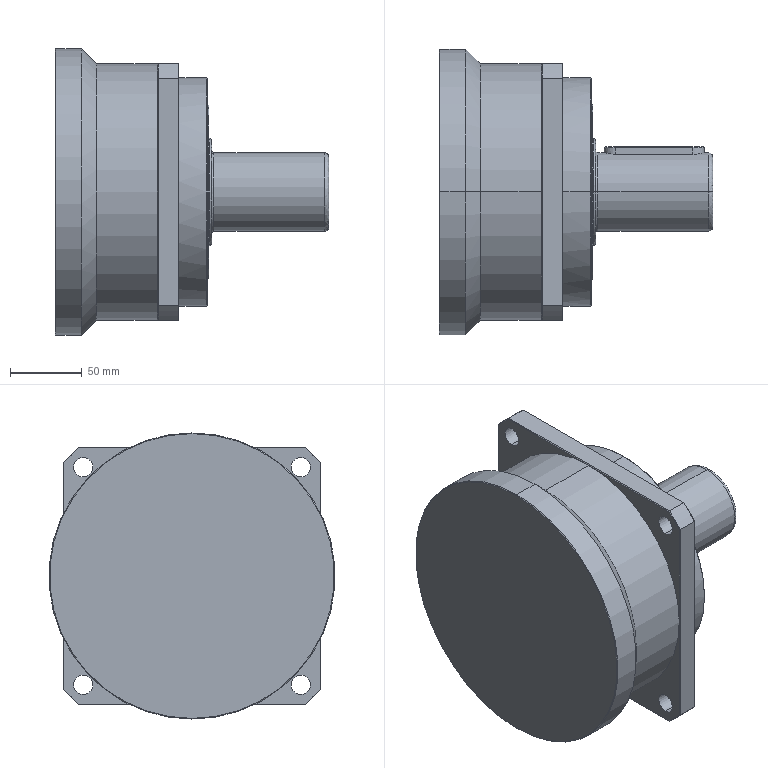Part | SolidWorks | features BaseBody 1 | 1 solid | 195 faces | box 191.495 x 200 x 200 mm | volume 3024344 mm3 | cylinder 94 | plane 54 | cone 41 | spline 6 | commonest cylinder face diameters 4 x40 78 x9 96 x9 6 x8 13.5 x8 240 x4